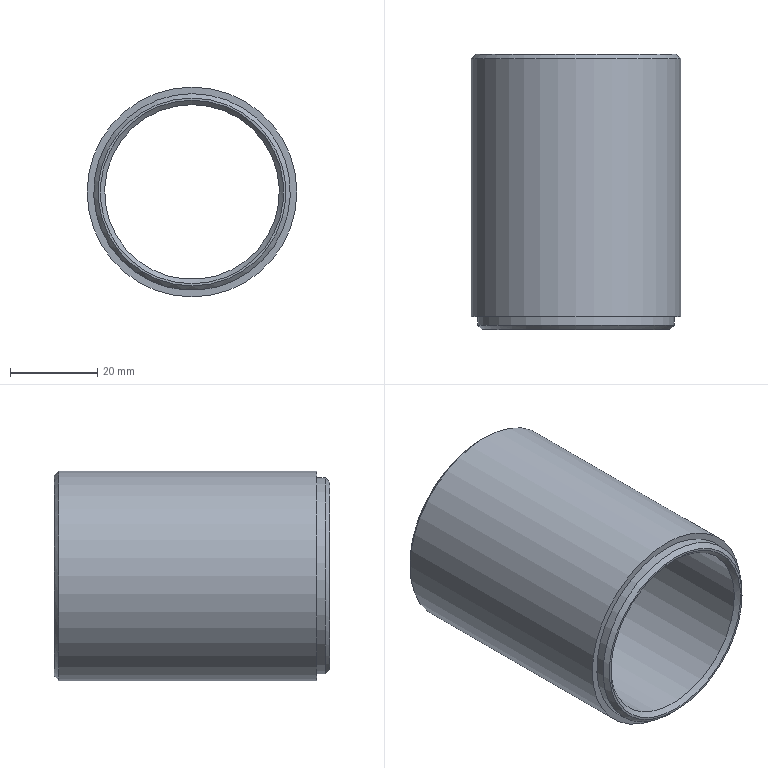Part | STEP file | JBJ-P-1013-04 | 1 solid | 10 faces | box 48 x 63 x 48 mm | volume 33905 mm3 | cone 4 | plane 3 | cylinder 3 | commonest cylinder face diameters 40 x1 45 x1 48 x1
STEP:
#1=CARTESIAN_POINT('',(0.,0.,21.5));
#2=VERTEX_POINT('',#1);
#3=CARTESIAN_POINT('',(0.,0.,0.));
#4=DIRECTION('',(0.,-1.,0.));
#5=DIRECTION('',(0.,0.,1.));
#6=AXIS2_PLACEMENT_3D('',#3,#4,#5);
#7=CIRCLE('',#6,21.5);
#8=EDGE_CURVE('',#2,#2,#7,.T.);
#9=ORIENTED_EDGE('',*,*,#8,.T.);
#10=EDGE_LOOP('',(#9));
#11=FACE_OUTER_BOUND('',#10,.T.);
#12=CARTESIAN_POINT('',(0.,0.,21.));
#13=VERTEX_POINT('',#12);
#14=CARTESIAN_POINT('',(0.,0.,0.));
#15=DIRECTION('',(0.,1.,0.));
#16=DIRECTION('',(0.,0.,1.));
#17=AXIS2_PLACEMENT_3D('',#14,#15,#16);
#18=CIRCLE('',#17,21.);
#19=EDGE_CURVE('',#13,#13,#18,.T.);
#20=ORIENTED_EDGE('',*,*,#19,.T.);
#21=EDGE_LOOP('',(#20));
#22=FACE_BOUND('',#21,.T.);
#23=CARTESIAN_POINT('',(0.,0.,0.));
#24=DIRECTION('',(0.,1.,0.));
#25=DIRECTION('',(0.,0.,1.));
#26=AXIS2_PLACEMENT_3D('',#23,#24,#25);
#27=PLANE('',#26);
#28=ADVANCED_FACE('',(#11,#22),#27,.F.);
#29=CARTESIAN_POINT('',(0.,1.,22.5));
#30=VERTEX_POINT('',#29);
#31=CARTESIAN_POINT('',(0.,1.,0.));
#32=DIRECTION('',(0.,1.,0.));
#33=DIRECTION('',(0.,0.,1.));
#34=AXIS2_PLACEMENT_3D('',#31,#32,#33);
#35=CIRCLE('',#34,22.5);
#36=EDGE_CURVE('',#30,#30,#35,.T.);
#37=ORIENTED_EDGE('',*,*,#36,.T.);
#38=EDGE_LOOP('',(#37));
#39=FACE_OUTER_BOUND('',#38,.T.);
#40=CARTESIAN_POINT('',(0.,3.,22.5));
#41=VERTEX_POINT('',#40);
#42=CARTESIAN_POINT('',(0.,3.,0.));
#43=DIRECTION('',(0.,1.,0.));
#44=DIRECTION('',(0.,0.,1.));
#45=AXIS2_PLACEMENT_3D('',#42,#43,#44);
#46=CIRCLE('',#45,22.5);
#47=EDGE_CURVE('',#41,#41,#46,.T.);
#48=ORIENTED_EDGE('',*,*,#47,.F.);
#49=EDGE_LOOP('',(#48));
#50=FACE_OUTER_BOUND('',#49,.T.);
#51=CARTESIAN_POINT('',(0.,3.,0.));
#52=DIRECTION('',(0.,-1.,0.));
#53=DIRECTION('',(0.,0.,-1.));
#54=AXIS2_PLACEMENT_3D('',#51,#52,#53);
#55=CYLINDRICAL_SURFACE('',#54,22.5);
#56=ADVANCED_FACE('',(#39,#50),#55,.T.);
#57=CARTESIAN_POINT('',(0.,62.,20.));
#58=VERTEX_POINT('',#57);
#59=CARTESIAN_POINT('',(0.,62.,0.));
#60=DIRECTION('',(0.,1.,0.));
#61=DIRECTION('',(0.,0.,1.));
#62=AXIS2_PLACEMENT_3D('',#59,#60,#61);
#63=CIRCLE('',#62,20.);
#64=EDGE_CURVE('',#58,#58,#63,.T.);
#65=ORIENTED_EDGE('',*,*,#64,.T.);
#66=EDGE_LOOP('',(#65));
#67=FACE_OUTER_BOUND('',#66,.T.);
#68=CARTESIAN_POINT('',(0.,1.,20.));
#69=VERTEX_POINT('',#68);
#70=CARTESIAN_POINT('',(0.,1.,0.));
#71=DIRECTION('',(0.,-1.,0.));
#72=DIRECTION('',(0.,0.,1.));
#73=AXIS2_PLACEMENT_3D('',#70,#71,#72);
#74=CIRCLE('',#73,20.);
#75=EDGE_CURVE('',#69,#69,#74,.T.);
#76=ORIENTED_EDGE('',*,*,#75,.T.);
#77=EDGE_LOOP('',(#76));
#78=FACE_OUTER_BOUND('',#77,.T.);
#79=CARTESIAN_POINT('',(0.,3.,0.));
#80=DIRECTION('',(0.,-1.,0.));
#81=DIRECTION('',(0.,0.,-1.));
#82=AXIS2_PLACEMENT_3D('',#79,#80,#81);
#83=CYLINDRICAL_SURFACE('',#82,20.);
#84=ADVANCED_FACE('',(#67,#78),#83,.F.);
#85=CARTESIAN_POINT('',(0.,63.,21.));
#86=VERTEX_POINT('',#85);
#87=CARTESIAN_POINT('',(0.,63.,0.));
#88=DIRECTION('',(0.,-1.,0.));
#89=DIRECTION('',(0.,0.,1.));
#90=AXIS2_PLACEMENT_3D('',#87,#88,#89);
#91=CIRCLE('',#90,21.);
#92=EDGE_CURVE('',#86,#86,#91,.T.);
#93=ORIENTED_EDGE('',*,*,#92,.T.);
#94=EDGE_LOOP('',(#93));
#95=FACE_BOUND('',#94,.T.);
#96=CARTESIAN_POINT('',(0.,63.,23.));
#97=VERTEX_POINT('',#96);
#98=CARTESIAN_POINT('',(0.,63.,0.));
#99=DIRECTION('',(0.,1.,0.));
#100=DIRECTION('',(0.,0.,1.));
#101=AXIS2_PLACEMENT_3D('',#98,#99,#100);
#102=CIRCLE('',#101,23.);
#103=EDGE_CURVE('',#97,#97,#102,.T.);
#104=ORIENTED_EDGE('',*,*,#103,.T.);
#105=EDGE_LOOP('',(#104));
#106=FACE_OUTER_BOUND('',#105,.T.);
#107=CARTESIAN_POINT('',(0.,63.,0.));
#108=DIRECTION('',(0.,1.,0.));
#109=DIRECTION('',(0.,0.,1.));
#110=AXIS2_PLACEMENT_3D('',#107,#108,#109);
#111=PLANE('',#110);
#112=ADVANCED_FACE('',(#95,#106),#111,.T.);
#113=ORIENTED_EDGE('',*,*,#47,.T.);
#114=EDGE_LOOP('',(#113));
#115=FACE_BOUND('',#114,.T.);
#116=CARTESIAN_POINT('',(0.,3.,24.));
#117=VERTEX_POINT('',#116);
#118=CARTESIAN_POINT('',(0.,3.,0.));
#119=DIRECTION('',(0.,1.,0.));
#120=DIRECTION('',(0.,0.,1.));
#121=AXIS2_PLACEMENT_3D('',#118,#119,#120);
#122=CIRCLE('',#121,24.);
#123=EDGE_CURVE('',#117,#117,#122,.T.);
#124=ORIENTED_EDGE('',*,*,#123,.F.);
#125=EDGE_LOOP('',(#124));
#126=FACE_OUTER_BOUND('',#125,.T.);
#127=CARTESIAN_POINT('',(0.,3.,0.));
#128=DIRECTION('',(0.,1.,0.));
#129=DIRECTION('',(0.,0.,1.));
#130=AXIS2_PLACEMENT_3D('',#127,#128,#129);
#131=PLANE('',#130);
#132=ADVANCED_FACE('',(#115,#126),#131,.F.);
#133=CARTESIAN_POINT('',(0.,62.,24.));
#134=VERTEX_POINT('',#133);
#135=CARTESIAN_POINT('',(0.,62.,0.));
#136=DIRECTION('',(0.,-1.,0.));
#137=DIRECTION('',(0.,0.,1.));
#138=AXIS2_PLACEMENT_3D('',#135,#136,#137);
#139=CIRCLE('',#138,24.);
#140=EDGE_CURVE('',#134,#134,#139,.T.);
#141=ORIENTED_EDGE('',*,*,#140,.T.);
#142=EDGE_LOOP('',(#141));
#143=FACE_OUTER_BOUND('',#142,.T.);
#144=ORIENTED_EDGE('',*,*,#123,.T.);
#145=EDGE_LOOP('',(#144));
#146=FACE_OUTER_BOUND('',#145,.T.);
#147=CARTESIAN_POINT('',(0.,63.,0.));
#148=DIRECTION('',(0.,-1.,0.));
#149=DIRECTION('',(0.,0.,-1.));
#150=AXIS2_PLACEMENT_3D('',#147,#148,#149);
#151=CYLINDRICAL_SURFACE('',#150,24.);
#152=ADVANCED_FACE('',(#143,#146),#151,.T.);
#153=ORIENTED_EDGE('',*,*,#92,.F.);
#154=EDGE_LOOP('',(#153));
#155=FACE_OUTER_BOUND('',#154,.T.);
#156=ORIENTED_EDGE('',*,*,#64,.F.);
#157=EDGE_LOOP('',(#156));
#158=FACE_BOUND('',#157,.T.);
#159=CARTESIAN_POINT('',(0.,62.,0.));
#160=DIRECTION('',(0.,1.,0.));
#161=DIRECTION('',(0.,0.,1.));
#162=AXIS2_PLACEMENT_3D('',#159,#160,#161);
#163=CONICAL_SURFACE('',#162,20.,0.7854);
#164=ADVANCED_FACE('',(#155,#158),#163,.F.);
#165=ORIENTED_EDGE('',*,*,#140,.F.);
#166=EDGE_LOOP('',(#165));
#167=FACE_OUTER_BOUND('',#166,.T.);
#168=ORIENTED_EDGE('',*,*,#103,.F.);
#169=EDGE_LOOP('',(#168));
#170=FACE_BOUND('',#169,.T.);
#171=CARTESIAN_POINT('',(0.,63.,0.));
#172=DIRECTION('',(0.,-1.,0.));
#173=DIRECTION('',(0.,0.,-1.));
#174=AXIS2_PLACEMENT_3D('',#171,#172,#173);
#175=CONICAL_SURFACE('',#174,23.,0.7854);
#176=ADVANCED_FACE('',(#167,#170),#175,.T.);
#177=ORIENTED_EDGE('',*,*,#8,.F.);
#178=EDGE_LOOP('',(#177));
#179=FACE_BOUND('',#178,.T.);
#180=ORIENTED_EDGE('',*,*,#36,.F.);
#181=EDGE_LOOP('',(#180));
#182=FACE_OUTER_BOUND('',#181,.T.);
#183=CARTESIAN_POINT('',(0.,1.,0.));
#184=DIRECTION('',(0.,1.,0.));
#185=DIRECTION('',(0.,0.,1.));
#186=AXIS2_PLACEMENT_3D('',#183,#184,#185);
#187=CONICAL_SURFACE('',#186,22.5,0.7854);
#188=ADVANCED_FACE('',(#179,#182),#187,.T.);
#189=ORIENTED_EDGE('',*,*,#75,.F.);
#190=EDGE_LOOP('',(#189));
#191=FACE_BOUND('',#190,.T.);
#192=ORIENTED_EDGE('',*,*,#19,.F.);
#193=EDGE_LOOP('',(#192));
#194=FACE_OUTER_BOUND('',#193,.T.);
#195=CARTESIAN_POINT('',(0.,0.,0.));
#196=DIRECTION('',(0.,-1.,0.));
#197=DIRECTION('',(0.,0.,-1.));
#198=AXIS2_PLACEMENT_3D('',#195,#196,#197);
#199=CONICAL_SURFACE('',#198,21.,0.7854);
#200=ADVANCED_FACE('',(#191,#194),#199,.F.);
#201=CLOSED_SHELL('',(#28,#56,#84,#112,#132,#152,#164,#176,#188,#200));
#202=MANIFOLD_SOLID_BREP('',#201);
#203=CARTESIAN_POINT('',(0.,0.,0.));
#204=DIRECTION('',(0.,0.,1.));
#205=DIRECTION('',(1.,0.,0.));
#206=AXIS2_PLACEMENT_3D('',#203,#204,#205);
#207=(LENGTH_UNIT()NAMED_UNIT(*)SI_UNIT(.MILLI.,.METRE.));
#208=UNCERTAINTY_MEASURE_WITH_UNIT(LENGTH_MEASURE(0.00001),#207,'','');
#209=(NAMED_UNIT(*)PLANE_ANGLE_UNIT()SI_UNIT($,.RADIAN.));
#210=(NAMED_UNIT(*)SI_UNIT($,.STERADIAN.)SOLID_ANGLE_UNIT());
#211=(GEOMETRIC_REPRESENTATION_CONTEXT(3)GLOBAL_UNCERTAINTY_ASSIGNED_CONTEXT((#208))GLOBAL_UNIT_ASSIGNED_CONTEXT((#207,#209,#210))REPRESENTATION_CONTEXT('',''));
#212=ADVANCED_BREP_SHAPE_REPRESENTATION('',(#202,#206),#211);